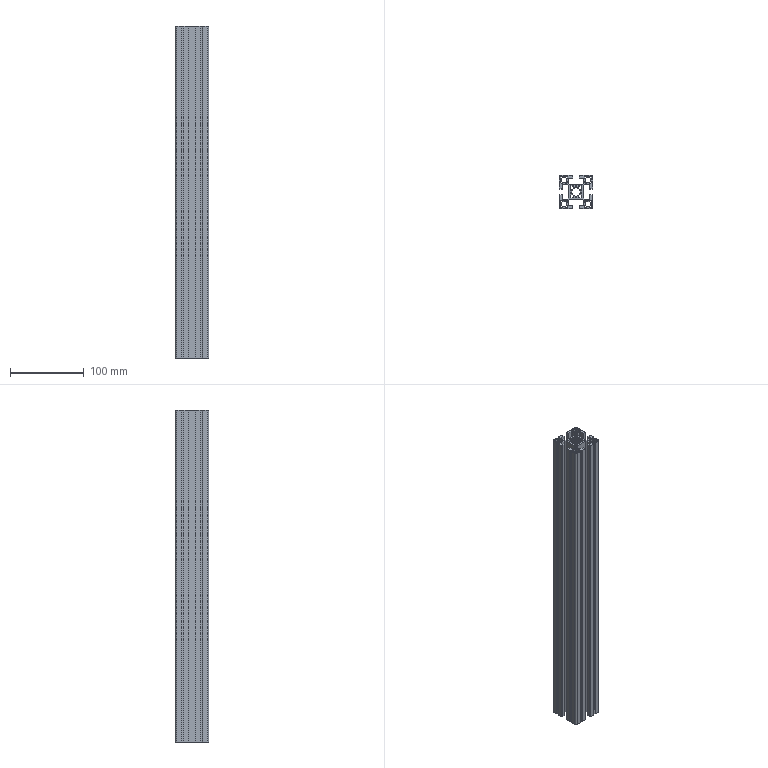Part | STEP file | 4545 profile 1 | 1 solid | 262 faces | box 45 x 45 x 450 mm | volume 312231 mm3 | plane 186 | cylinder 76 | commonest cylinder face diameters 2 x44 8 x20 12 x8 4 x4